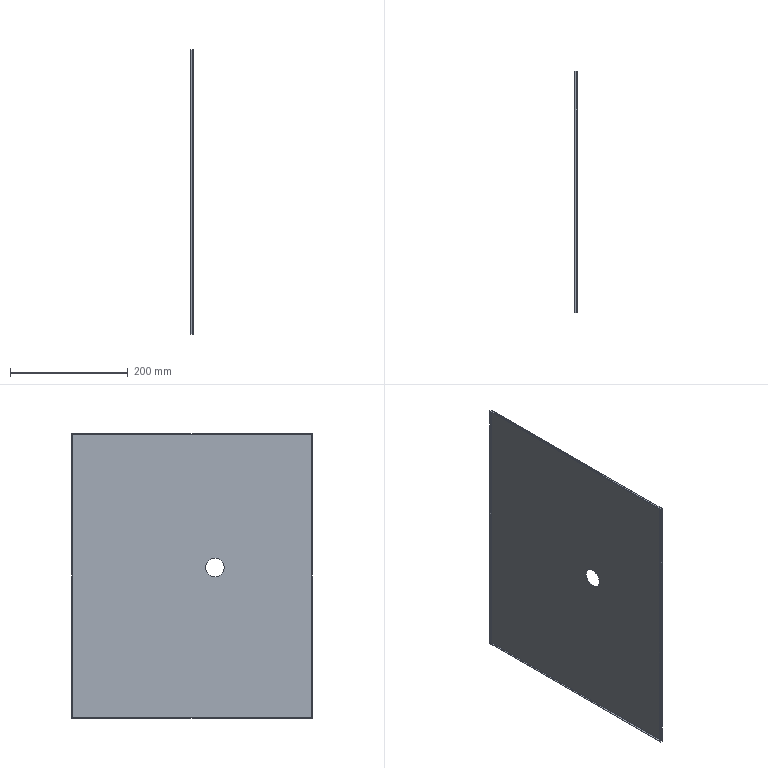Part | STEP file | 09-30 Cover base plate | 1 solid | 13 faces | box 4 x 410 x 485 mm | volume 203404 mm3 | plane 11 | cylinder 2 | commonest cylinder face diameters 32 x2
STEP:
#1=CARTESIAN_POINT('',(0.,0.,0.));
#2=DIRECTION('',(0.,0.,1.));
#3=DIRECTION('',(1.,0.,0.));
#4=AXIS2_PLACEMENT_3D('',#1,#2,#3);
#5=CARTESIAN_POINT('',(1.,-39.,30.5));
#6=VERTEX_POINT('',#5);
#7=CARTESIAN_POINT('',(0.,-39.,30.5));
#8=VERTEX_POINT('',#7);
#9=CARTESIAN_POINT('',(1.,-39.,30.5));
#10=DIRECTION('',(-1.,0.,0.));
#11=VECTOR('',#10,1.);
#12=LINE('',#9,#11);
#13=CARTESIAN_POINT('',(1.,-39.,14.5));
#14=DIRECTION('',(-1.,0.,0.));
#15=DIRECTION('',(0.,0.,1.));
#16=AXIS2_PLACEMENT_3D('',#13,#14,#15);
#17=CYLINDRICAL_SURFACE('',#16,16.);
#18=CARTESIAN_POINT('',(6.283,0.));
#19=DIRECTION('',(0.,1.));
#20=VECTOR('',#19,1.);
#21=LINE('',#18,#20);
#22=(GEOMETRIC_REPRESENTATION_CONTEXT(2)PARAMETRIC_REPRESENTATION_CONTEXT()REPRESENTATION_CONTEXT('',''));
#23=DEFINITIONAL_REPRESENTATION('',(#21),#22);
#24=PCURVE('',#17,#23);
#25=CARTESIAN_POINT('',(1.,-39.,14.5));
#26=DIRECTION('',(-1.,0.,0.));
#27=DIRECTION('',(0.,0.,1.));
#28=AXIS2_PLACEMENT_3D('',#25,#26,#27);
#29=CYLINDRICAL_SURFACE('',#28,16.);
#30=CARTESIAN_POINT('',(0.,0.));
#31=DIRECTION('',(0.,1.));
#32=VECTOR('',#31,1.);
#33=LINE('',#30,#32);
#34=(GEOMETRIC_REPRESENTATION_CONTEXT(2)PARAMETRIC_REPRESENTATION_CONTEXT()REPRESENTATION_CONTEXT('',''));
#35=DEFINITIONAL_REPRESENTATION('',(#33),#34);
#36=PCURVE('',#29,#35);
#37=SURFACE_CURVE('',#12,(#24,#36),.PCURVE_S1.);
#38=EDGE_CURVE('',#6,#8,#37,.T.);
#39=ORIENTED_EDGE('',*,*,#38,.T.);
#40=CARTESIAN_POINT('',(0.,-39.,-1.5));
#41=VERTEX_POINT('',#40);
#42=CARTESIAN_POINT('',(0.,-39.,14.5));
#43=DIRECTION('',(-1.,0.,0.));
#44=DIRECTION('',(0.,0.,1.));
#45=AXIS2_PLACEMENT_3D('',#42,#43,#44);
#46=CIRCLE('',#45,16.);
#47=CARTESIAN_POINT('',(0.,1.));
#48=DIRECTION('',(1.,0.));
#49=VECTOR('',#48,1.);
#50=LINE('',#47,#49);
#51=(GEOMETRIC_REPRESENTATION_CONTEXT(2)PARAMETRIC_REPRESENTATION_CONTEXT()REPRESENTATION_CONTEXT('',''));
#52=DEFINITIONAL_REPRESENTATION('',(#50),#51);
#53=PCURVE('',#17,#52);
#54=CARTESIAN_POINT('',(0.,-204.,-241.5));
#55=DIRECTION('',(-1.,0.,0.));
#56=DIRECTION('',(0.,0.,1.));
#57=AXIS2_PLACEMENT_3D('',#54,#55,#56);
#58=PLANE('',#57);
#59=CARTESIAN_POINT('',(256.,165.));
#60=DIRECTION('',(1.,0.));
#61=AXIS2_PLACEMENT_2D('',#59,#60);
#62=CIRCLE('',#61,16.);
#63=(GEOMETRIC_REPRESENTATION_CONTEXT(2)PARAMETRIC_REPRESENTATION_CONTEXT()REPRESENTATION_CONTEXT('',''));
#64=DEFINITIONAL_REPRESENTATION('',(#62),#63);
#65=PCURVE('',#58,#64);
#66=SURFACE_CURVE('',#46,(#53,#65),.PCURVE_S1.);
#67=EDGE_CURVE('',#41,#8,#66,.T.);
#68=ORIENTED_EDGE('',*,*,#67,.F.);
#69=CARTESIAN_POINT('',(1.,-39.,-1.5));
#70=VERTEX_POINT('',#69);
#71=CARTESIAN_POINT('',(1.,-39.,-1.5));
#72=DIRECTION('',(-1.,0.,0.));
#73=VECTOR('',#72,1.);
#74=LINE('',#71,#73);
#75=CARTESIAN_POINT('',(3.142,0.));
#76=DIRECTION('',(0.,1.));
#77=VECTOR('',#76,1.);
#78=LINE('',#75,#77);
#79=(GEOMETRIC_REPRESENTATION_CONTEXT(2)PARAMETRIC_REPRESENTATION_CONTEXT()REPRESENTATION_CONTEXT('',''));
#80=DEFINITIONAL_REPRESENTATION('',(#78),#79);
#81=PCURVE('',#17,#80);
#82=CARTESIAN_POINT('',(3.142,0.));
#83=DIRECTION('',(0.,1.));
#84=VECTOR('',#83,1.);
#85=LINE('',#82,#84);
#86=(GEOMETRIC_REPRESENTATION_CONTEXT(2)PARAMETRIC_REPRESENTATION_CONTEXT()REPRESENTATION_CONTEXT('',''));
#87=DEFINITIONAL_REPRESENTATION('',(#85),#86);
#88=PCURVE('',#29,#87);
#89=SURFACE_CURVE('',#74,(#81,#88),.PCURVE_S1.);
#90=EDGE_CURVE('',#70,#41,#89,.T.);
#91=ORIENTED_EDGE('',*,*,#90,.F.);
#92=CARTESIAN_POINT('',(1.,-39.,14.5));
#93=DIRECTION('',(1.,0.,0.));
#94=DIRECTION('',(0.,0.,1.));
#95=AXIS2_PLACEMENT_3D('',#92,#93,#94);
#96=CIRCLE('',#95,16.);
#97=CARTESIAN_POINT('',(6.283,0.));
#98=DIRECTION('',(-1.,0.));
#99=VECTOR('',#98,1.);
#100=LINE('',#97,#99);
#101=(GEOMETRIC_REPRESENTATION_CONTEXT(2)PARAMETRIC_REPRESENTATION_CONTEXT()REPRESENTATION_CONTEXT('',''));
#102=DEFINITIONAL_REPRESENTATION('',(#100),#101);
#103=PCURVE('',#17,#102);
#104=CARTESIAN_POINT('',(1.,-205.,-242.5));
#105=DIRECTION('',(-1.,0.,0.));
#106=DIRECTION('',(0.,0.,1.));
#107=AXIS2_PLACEMENT_3D('',#104,#105,#106);
#108=PLANE('',#107);
#109=CARTESIAN_POINT('',(273.,166.));
#110=CARTESIAN_POINT('',(273.,138.287));
#111=CARTESIAN_POINT('',(249.,152.144));
#112=CARTESIAN_POINT('',(225.,166.));
#113=CARTESIAN_POINT('',(249.,179.856));
#114=CARTESIAN_POINT('',(273.,193.713));
#115=CARTESIAN_POINT('',(273.,166.));
#116=(BOUNDED_CURVE()B_SPLINE_CURVE(2,(#109,#110,#111,#112,#113,#114,#115),.UNSPECIFIED.,.T.,.F.)B_SPLINE_CURVE_WITH_KNOTS((1,2,2,2,2,1),(-2.094,0.,2.094,4.189,6.283,8.378),.UNSPECIFIED.)CURVE()GEOMETRIC_REPRESENTATION_ITEM()RATIONAL_B_SPLINE_CURVE((1.,0.5,1.,0.5,1.,0.5,1.))REPRESENTATION_ITEM(''));
#117=(GEOMETRIC_REPRESENTATION_CONTEXT(2)PARAMETRIC_REPRESENTATION_CONTEXT()REPRESENTATION_CONTEXT('',''));
#118=DEFINITIONAL_REPRESENTATION('',(#116),#117);
#119=PCURVE('',#108,#118);
#120=SURFACE_CURVE('',#96,(#103,#119),.PCURVE_S1.);
#121=EDGE_CURVE('',#6,#70,#120,.T.);
#122=ORIENTED_EDGE('',*,*,#121,.F.);
#123=EDGE_LOOP('',(#39,#68,#91,#122));
#124=FACE_BOUND('',#123,.F.);
#125=ADVANCED_FACE('',(#124),#17,.F.);
#126=CARTESIAN_POINT('',(0.,-39.,14.5));
#127=DIRECTION('',(-1.,0.,0.));
#128=DIRECTION('',(0.,0.,1.));
#129=AXIS2_PLACEMENT_3D('',#126,#127,#128);
#130=CIRCLE('',#129,16.);
#131=CARTESIAN_POINT('',(0.,1.));
#132=DIRECTION('',(1.,0.));
#133=VECTOR('',#132,1.);
#134=LINE('',#131,#133);
#135=(GEOMETRIC_REPRESENTATION_CONTEXT(2)PARAMETRIC_REPRESENTATION_CONTEXT()REPRESENTATION_CONTEXT('',''));
#136=DEFINITIONAL_REPRESENTATION('',(#134),#135);
#137=PCURVE('',#29,#136);
#138=CARTESIAN_POINT('',(256.,165.));
#139=DIRECTION('',(1.,0.));
#140=AXIS2_PLACEMENT_2D('',#138,#139);
#141=CIRCLE('',#140,16.);
#142=(GEOMETRIC_REPRESENTATION_CONTEXT(2)PARAMETRIC_REPRESENTATION_CONTEXT()REPRESENTATION_CONTEXT('',''));
#143=DEFINITIONAL_REPRESENTATION('',(#141),#142);
#144=PCURVE('',#58,#143);
#145=SURFACE_CURVE('',#130,(#137,#144),.PCURVE_S1.);
#146=EDGE_CURVE('',#8,#41,#145,.T.);
#147=ORIENTED_EDGE('',*,*,#146,.F.);
#148=ORIENTED_EDGE('',*,*,#38,.F.);
#149=CARTESIAN_POINT('',(1.,-39.,14.5));
#150=DIRECTION('',(1.,0.,0.));
#151=DIRECTION('',(0.,0.,1.));
#152=AXIS2_PLACEMENT_3D('',#149,#150,#151);
#153=CIRCLE('',#152,16.);
#154=CARTESIAN_POINT('',(6.283,0.));
#155=DIRECTION('',(-1.,0.));
#156=VECTOR('',#155,1.);
#157=LINE('',#154,#156);
#158=(GEOMETRIC_REPRESENTATION_CONTEXT(2)PARAMETRIC_REPRESENTATION_CONTEXT()REPRESENTATION_CONTEXT('',''));
#159=DEFINITIONAL_REPRESENTATION('',(#157),#158);
#160=PCURVE('',#29,#159);
#161=CARTESIAN_POINT('',(273.,166.));
#162=CARTESIAN_POINT('',(273.,138.287));
#163=CARTESIAN_POINT('',(249.,152.144));
#164=CARTESIAN_POINT('',(225.,166.));
#165=CARTESIAN_POINT('',(249.,179.856));
#166=CARTESIAN_POINT('',(273.,193.713));
#167=CARTESIAN_POINT('',(273.,166.));
#168=(BOUNDED_CURVE()B_SPLINE_CURVE(2,(#161,#162,#163,#164,#165,#166,#167),.UNSPECIFIED.,.T.,.F.)B_SPLINE_CURVE_WITH_KNOTS((1,2,2,2,2,1),(-2.094,0.,2.094,4.189,6.283,8.378),.UNSPECIFIED.)CURVE()GEOMETRIC_REPRESENTATION_ITEM()RATIONAL_B_SPLINE_CURVE((1.,0.5,1.,0.5,1.,0.5,1.))REPRESENTATION_ITEM(''));
#169=(GEOMETRIC_REPRESENTATION_CONTEXT(2)PARAMETRIC_REPRESENTATION_CONTEXT()REPRESENTATION_CONTEXT('',''));
#170=DEFINITIONAL_REPRESENTATION('',(#168),#169);
#171=PCURVE('',#108,#170);
#172=SURFACE_CURVE('',#153,(#160,#171),.PCURVE_S1.);
#173=EDGE_CURVE('',#70,#6,#172,.T.);
#174=ORIENTED_EDGE('',*,*,#173,.F.);
#175=ORIENTED_EDGE('',*,*,#90,.T.);
#176=EDGE_LOOP('',(#147,#148,#174,#175));
#177=FACE_BOUND('',#176,.F.);
#178=ADVANCED_FACE('',(#177),#29,.F.);
#179=ORIENTED_EDGE('',*,*,#146,.F.);
#180=ORIENTED_EDGE('',*,*,#67,.F.);
#181=EDGE_LOOP('',(#179,#180));
#182=FACE_BOUND('',#181,.T.);
#183=CARTESIAN_POINT('',(0.,204.,-241.5));
#184=VERTEX_POINT('',#183);
#185=CARTESIAN_POINT('',(0.,-204.,-241.5));
#186=VERTEX_POINT('',#185);
#187=CARTESIAN_POINT('',(0.,0.,-241.5));
#188=DIRECTION('',(0.,-1.,0.));
#189=VECTOR('',#188,1.);
#190=LINE('',#187,#189);
#191=CARTESIAN_POINT('',(0.,204.));
#192=DIRECTION('',(0.,-1.));
#193=VECTOR('',#192,1.);
#194=LINE('',#191,#193);
#195=(GEOMETRIC_REPRESENTATION_CONTEXT(2)PARAMETRIC_REPRESENTATION_CONTEXT()REPRESENTATION_CONTEXT('',''));
#196=DEFINITIONAL_REPRESENTATION('',(#194),#195);
#197=PCURVE('',#58,#196);
#198=CARTESIAN_POINT('',(-3.,-204.,-241.5));
#199=DIRECTION('',(0.,0.,1.));
#200=DIRECTION('',(1.,0.,0.));
#201=AXIS2_PLACEMENT_3D('',#198,#199,#200);
#202=PLANE('',#201);
#203=CARTESIAN_POINT('',(3.,204.));
#204=DIRECTION('',(0.,-1.));
#205=VECTOR('',#204,1.);
#206=LINE('',#203,#205);
#207=(GEOMETRIC_REPRESENTATION_CONTEXT(2)PARAMETRIC_REPRESENTATION_CONTEXT()REPRESENTATION_CONTEXT('',''));
#208=DEFINITIONAL_REPRESENTATION('',(#206),#207);
#209=PCURVE('',#202,#208);
#210=SURFACE_CURVE('',#190,(#197,#209),.PCURVE_S1.);
#211=EDGE_CURVE('',#184,#186,#210,.T.);
#212=ORIENTED_EDGE('',*,*,#211,.T.);
#213=CARTESIAN_POINT('',(0.,-204.,241.5));
#214=VERTEX_POINT('',#213);
#215=CARTESIAN_POINT('',(0.,-204.,0.));
#216=DIRECTION('',(0.,0.,1.));
#217=VECTOR('',#216,1.);
#218=LINE('',#215,#217);
#219=CARTESIAN_POINT('',(241.5,0.));
#220=DIRECTION('',(1.,0.));
#221=VECTOR('',#220,1.);
#222=LINE('',#219,#221);
#223=(GEOMETRIC_REPRESENTATION_CONTEXT(2)PARAMETRIC_REPRESENTATION_CONTEXT()REPRESENTATION_CONTEXT('',''));
#224=DEFINITIONAL_REPRESENTATION('',(#222),#223);
#225=PCURVE('',#58,#224);
#226=CARTESIAN_POINT('',(-3.,-204.,-241.5));
#227=DIRECTION('',(0.,1.,0.));
#228=DIRECTION('',(0.,0.,1.));
#229=AXIS2_PLACEMENT_3D('',#226,#227,#228);
#230=PLANE('',#229);
#231=CARTESIAN_POINT('',(241.5,3.));
#232=DIRECTION('',(1.,0.));
#233=VECTOR('',#232,1.);
#234=LINE('',#231,#233);
#235=(GEOMETRIC_REPRESENTATION_CONTEXT(2)PARAMETRIC_REPRESENTATION_CONTEXT()REPRESENTATION_CONTEXT('',''));
#236=DEFINITIONAL_REPRESENTATION('',(#234),#235);
#237=PCURVE('',#230,#236);
#238=SURFACE_CURVE('',#218,(#225,#237),.PCURVE_S1.);
#239=EDGE_CURVE('',#186,#214,#238,.T.);
#240=ORIENTED_EDGE('',*,*,#239,.T.);
#241=CARTESIAN_POINT('',(0.,204.,241.5));
#242=VERTEX_POINT('',#241);
#243=CARTESIAN_POINT('',(0.,0.,241.5));
#244=DIRECTION('',(0.,1.,0.));
#245=VECTOR('',#244,1.);
#246=LINE('',#243,#245);
#247=CARTESIAN_POINT('',(483.,204.));
#248=DIRECTION('',(0.,1.));
#249=VECTOR('',#248,1.);
#250=LINE('',#247,#249);
#251=(GEOMETRIC_REPRESENTATION_CONTEXT(2)PARAMETRIC_REPRESENTATION_CONTEXT()REPRESENTATION_CONTEXT('',''));
#252=DEFINITIONAL_REPRESENTATION('',(#250),#251);
#253=PCURVE('',#58,#252);
#254=CARTESIAN_POINT('',(0.,-204.,241.5));
#255=DIRECTION('',(0.,0.,-1.));
#256=DIRECTION('',(-1.,0.,0.));
#257=AXIS2_PLACEMENT_3D('',#254,#255,#256);
#258=PLANE('',#257);
#259=CARTESIAN_POINT('',(0.,204.));
#260=DIRECTION('',(0.,1.));
#261=VECTOR('',#260,1.);
#262=LINE('',#259,#261);
#263=(GEOMETRIC_REPRESENTATION_CONTEXT(2)PARAMETRIC_REPRESENTATION_CONTEXT()REPRESENTATION_CONTEXT('',''));
#264=DEFINITIONAL_REPRESENTATION('',(#262),#263);
#265=PCURVE('',#258,#264);
#266=SURFACE_CURVE('',#246,(#253,#265),.PCURVE_S1.);
#267=EDGE_CURVE('',#214,#242,#266,.T.);
#268=ORIENTED_EDGE('',*,*,#267,.T.);
#269=CARTESIAN_POINT('',(0.,204.,0.));
#270=DIRECTION('',(0.,0.,-1.));
#271=VECTOR('',#270,1.);
#272=LINE('',#269,#271);
#273=CARTESIAN_POINT('',(241.5,408.));
#274=DIRECTION('',(-1.,0.));
#275=VECTOR('',#274,1.);
#276=LINE('',#273,#275);
#277=(GEOMETRIC_REPRESENTATION_CONTEXT(2)PARAMETRIC_REPRESENTATION_CONTEXT()REPRESENTATION_CONTEXT('',''));
#278=DEFINITIONAL_REPRESENTATION('',(#276),#277);
#279=PCURVE('',#58,#278);
#280=CARTESIAN_POINT('',(-3.,204.,241.5));
#281=DIRECTION('',(0.,-1.,0.));
#282=DIRECTION('',(0.,0.,-1.));
#283=AXIS2_PLACEMENT_3D('',#280,#281,#282);
#284=PLANE('',#283);
#285=CARTESIAN_POINT('',(241.5,3.));
#286=DIRECTION('',(1.,0.));
#287=VECTOR('',#286,1.);
#288=LINE('',#285,#287);
#289=(GEOMETRIC_REPRESENTATION_CONTEXT(2)PARAMETRIC_REPRESENTATION_CONTEXT()REPRESENTATION_CONTEXT('',''));
#290=DEFINITIONAL_REPRESENTATION('',(#288),#289);
#291=PCURVE('',#284,#290);
#292=SURFACE_CURVE('',#272,(#279,#291),.PCURVE_S1.);
#293=EDGE_CURVE('',#242,#184,#292,.T.);
#294=ORIENTED_EDGE('',*,*,#293,.T.);
#295=EDGE_LOOP('',(#212,#240,#268,#294));
#296=FACE_BOUND('',#295,.T.);
#297=ADVANCED_FACE('',(#182,#296),#58,.T.);
#298=ORIENTED_EDGE('',*,*,#121,.F.);
#299=ORIENTED_EDGE('',*,*,#173,.F.);
#300=EDGE_LOOP('',(#298,#299));
#301=FACE_BOUND('',#300,.T.);
#302=CARTESIAN_POINT('',(1.,205.,242.5));
#303=VERTEX_POINT('',#302);
#304=CARTESIAN_POINT('',(1.,205.,-242.5));
#305=VERTEX_POINT('',#304);
#306=CARTESIAN_POINT('',(1.,205.,0.));
#307=DIRECTION('',(0.,0.,-1.));
#308=VECTOR('',#307,1.);
#309=LINE('',#306,#308);
#310=CARTESIAN_POINT('',(242.5,410.));
#311=DIRECTION('',(-1.,0.));
#312=VECTOR('',#311,1.);
#313=LINE('',#310,#312);
#314=(GEOMETRIC_REPRESENTATION_CONTEXT(2)PARAMETRIC_REPRESENTATION_CONTEXT()REPRESENTATION_CONTEXT('',''));
#315=DEFINITIONAL_REPRESENTATION('',(#313),#314);
#316=PCURVE('',#108,#315);
#317=CARTESIAN_POINT('',(-3.,205.,242.5));
#318=DIRECTION('',(0.,-1.,0.));
#319=DIRECTION('',(0.,0.,-1.));
#320=AXIS2_PLACEMENT_3D('',#317,#318,#319);
#321=PLANE('',#320);
#322=CARTESIAN_POINT('',(242.5,4.));
#323=DIRECTION('',(1.,0.));
#324=VECTOR('',#323,1.);
#325=LINE('',#322,#324);
#326=(GEOMETRIC_REPRESENTATION_CONTEXT(2)PARAMETRIC_REPRESENTATION_CONTEXT()REPRESENTATION_CONTEXT('',''));
#327=DEFINITIONAL_REPRESENTATION('',(#325),#326);
#328=PCURVE('',#321,#327);
#329=SURFACE_CURVE('',#309,(#316,#328),.PCURVE_S1.);
#330=EDGE_CURVE('',#303,#305,#329,.T.);
#331=ORIENTED_EDGE('',*,*,#330,.F.);
#332=CARTESIAN_POINT('',(1.,-205.,242.5));
#333=VERTEX_POINT('',#332);
#334=CARTESIAN_POINT('',(1.,0.,242.5));
#335=DIRECTION('',(0.,1.,0.));
#336=VECTOR('',#335,1.);
#337=LINE('',#334,#336);
#338=CARTESIAN_POINT('',(485.,205.));
#339=DIRECTION('',(0.,1.));
#340=VECTOR('',#339,1.);
#341=LINE('',#338,#340);
#342=(GEOMETRIC_REPRESENTATION_CONTEXT(2)PARAMETRIC_REPRESENTATION_CONTEXT()REPRESENTATION_CONTEXT('',''));
#343=DEFINITIONAL_REPRESENTATION('',(#341),#342);
#344=PCURVE('',#108,#343);
#345=CARTESIAN_POINT('',(1.,-205.,242.5));
#346=DIRECTION('',(0.,0.,-1.));
#347=DIRECTION('',(-1.,0.,0.));
#348=AXIS2_PLACEMENT_3D('',#345,#346,#347);
#349=PLANE('',#348);
#350=CARTESIAN_POINT('',(0.,205.));
#351=DIRECTION('',(0.,1.));
#352=VECTOR('',#351,1.);
#353=LINE('',#350,#352);
#354=(GEOMETRIC_REPRESENTATION_CONTEXT(2)PARAMETRIC_REPRESENTATION_CONTEXT()REPRESENTATION_CONTEXT('',''));
#355=DEFINITIONAL_REPRESENTATION('',(#353),#354);
#356=PCURVE('',#349,#355);
#357=SURFACE_CURVE('',#337,(#344,#356),.PCURVE_S1.);
#358=EDGE_CURVE('',#333,#303,#357,.T.);
#359=ORIENTED_EDGE('',*,*,#358,.F.);
#360=CARTESIAN_POINT('',(1.,-205.,-242.5));
#361=VERTEX_POINT('',#360);
#362=CARTESIAN_POINT('',(1.,-205.,0.));
#363=DIRECTION('',(0.,0.,1.));
#364=VECTOR('',#363,1.);
#365=LINE('',#362,#364);
#366=CARTESIAN_POINT('',(242.5,0.));
#367=DIRECTION('',(1.,0.));
#368=VECTOR('',#367,1.);
#369=LINE('',#366,#368);
#370=(GEOMETRIC_REPRESENTATION_CONTEXT(2)PARAMETRIC_REPRESENTATION_CONTEXT()REPRESENTATION_CONTEXT('',''));
#371=DEFINITIONAL_REPRESENTATION('',(#369),#370);
#372=PCURVE('',#108,#371);
#373=CARTESIAN_POINT('',(-3.,-205.,-242.5));
#374=DIRECTION('',(0.,1.,0.));
#375=DIRECTION('',(0.,0.,1.));
#376=AXIS2_PLACEMENT_3D('',#373,#374,#375);
#377=PLANE('',#376);
#378=CARTESIAN_POINT('',(242.5,4.));
#379=DIRECTION('',(1.,0.));
#380=VECTOR('',#379,1.);
#381=LINE('',#378,#380);
#382=(GEOMETRIC_REPRESENTATION_CONTEXT(2)PARAMETRIC_REPRESENTATION_CONTEXT()REPRESENTATION_CONTEXT('',''));
#383=DEFINITIONAL_REPRESENTATION('',(#381),#382);
#384=PCURVE('',#377,#383);
#385=SURFACE_CURVE('',#365,(#372,#384),.PCURVE_S1.);
#386=EDGE_CURVE('',#361,#333,#385,.T.);
#387=ORIENTED_EDGE('',*,*,#386,.F.);
#388=CARTESIAN_POINT('',(1.,0.,-242.5));
#389=DIRECTION('',(0.,-1.,0.));
#390=VECTOR('',#389,1.);
#391=LINE('',#388,#390);
#392=CARTESIAN_POINT('',(0.,205.));
#393=DIRECTION('',(0.,-1.));
#394=VECTOR('',#393,1.);
#395=LINE('',#392,#394);
#396=(GEOMETRIC_REPRESENTATION_CONTEXT(2)PARAMETRIC_REPRESENTATION_CONTEXT()REPRESENTATION_CONTEXT('',''));
#397=DEFINITIONAL_REPRESENTATION('',(#395),#396);
#398=PCURVE('',#108,#397);
#399=CARTESIAN_POINT('',(-3.,-205.,-242.5));
#400=DIRECTION('',(0.,0.,1.));
#401=DIRECTION('',(1.,0.,0.));
#402=AXIS2_PLACEMENT_3D('',#399,#400,#401);
#403=PLANE('',#402);
#404=CARTESIAN_POINT('',(4.,205.));
#405=DIRECTION('',(0.,-1.));
#406=VECTOR('',#405,1.);
#407=LINE('',#404,#406);
#408=(GEOMETRIC_REPRESENTATION_CONTEXT(2)PARAMETRIC_REPRESENTATION_CONTEXT()REPRESENTATION_CONTEXT('',''));
#409=DEFINITIONAL_REPRESENTATION('',(#407),#408);
#410=PCURVE('',#403,#409);
#411=SURFACE_CURVE('',#391,(#398,#410),.PCURVE_S1.);
#412=EDGE_CURVE('',#305,#361,#411,.T.);
#413=ORIENTED_EDGE('',*,*,#412,.F.);
#414=EDGE_LOOP('',(#331,#359,#387,#413));
#415=FACE_BOUND('',#414,.T.);
#416=ADVANCED_FACE('',(#301,#415),#108,.F.);
#417=CARTESIAN_POINT('',(-3.,-204.,-241.5));
#418=VERTEX_POINT('',#417);
#419=CARTESIAN_POINT('',(-3.,-204.,241.5));
#420=VERTEX_POINT('',#419);
#421=CARTESIAN_POINT('',(-3.,-204.,0.));
#422=DIRECTION('',(0.,0.,1.));
#423=VECTOR('',#422,1.);
#424=LINE('',#421,#423);
#425=CARTESIAN_POINT('',(241.5,0.));
#426=DIRECTION('',(1.,0.));
#427=VECTOR('',#426,1.);
#428=LINE('',#425,#427);
#429=(GEOMETRIC_REPRESENTATION_CONTEXT(2)PARAMETRIC_REPRESENTATION_CONTEXT()REPRESENTATION_CONTEXT('',''));
#430=DEFINITIONAL_REPRESENTATION('',(#428),#429);
#431=PCURVE('',#230,#430);
#432=CARTESIAN_POINT('',(-3.,-205.,242.5));
#433=DIRECTION('',(1.,0.,0.));
#434=DIRECTION('',(0.,0.,-1.));
#435=AXIS2_PLACEMENT_3D('',#432,#433,#434);
#436=PLANE('',#435);
#437=CARTESIAN_POINT('',(242.5,1.));
#438=DIRECTION('',(-1.,0.));
#439=VECTOR('',#438,1.);
#440=LINE('',#437,#439);
#441=(GEOMETRIC_REPRESENTATION_CONTEXT(2)PARAMETRIC_REPRESENTATION_CONTEXT()REPRESENTATION_CONTEXT('',''));
#442=DEFINITIONAL_REPRESENTATION('',(#440),#441);
#443=PCURVE('',#436,#442);
#444=SURFACE_CURVE('',#424,(#431,#443),.PCURVE_S1.);
#445=EDGE_CURVE('',#418,#420,#444,.T.);
#446=ORIENTED_EDGE('',*,*,#445,.T.);
#447=CARTESIAN_POINT('',(-1.5,-204.,241.5));
#448=DIRECTION('',(1.,0.,0.));
#449=VECTOR('',#448,1.);
#450=LINE('',#447,#449);
#451=CARTESIAN_POINT('',(483.,1.5));
#452=DIRECTION('',(0.,1.));
#453=VECTOR('',#452,1.);
#454=LINE('',#451,#453);
#455=(GEOMETRIC_REPRESENTATION_CONTEXT(2)PARAMETRIC_REPRESENTATION_CONTEXT()REPRESENTATION_CONTEXT('',''));
#456=DEFINITIONAL_REPRESENTATION('',(#454),#455);
#457=PCURVE('',#230,#456);
#458=CARTESIAN_POINT('',(1.5,0.));
#459=DIRECTION('',(-1.,0.));
#460=VECTOR('',#459,1.);
#461=LINE('',#458,#460);
#462=(GEOMETRIC_REPRESENTATION_CONTEXT(2)PARAMETRIC_REPRESENTATION_CONTEXT()REPRESENTATION_CONTEXT('',''));
#463=DEFINITIONAL_REPRESENTATION('',(#461),#462);
#464=PCURVE('',#258,#463);
#465=SURFACE_CURVE('',#450,(#457,#464),.PCURVE_S1.);
#466=EDGE_CURVE('',#420,#214,#465,.T.);
#467=ORIENTED_EDGE('',*,*,#466,.T.);
#468=ORIENTED_EDGE('',*,*,#239,.F.);
#469=CARTESIAN_POINT('',(-1.5,-204.,-241.5));
#470=DIRECTION('',(-1.,0.,0.));
#471=VECTOR('',#470,1.);
#472=LINE('',#469,#471);
#473=CARTESIAN_POINT('',(0.,1.5));
#474=DIRECTION('',(0.,-1.));
#475=VECTOR('',#474,1.);
#476=LINE('',#473,#475);
#477=(GEOMETRIC_REPRESENTATION_CONTEXT(2)PARAMETRIC_REPRESENTATION_CONTEXT()REPRESENTATION_CONTEXT('',''));
#478=DEFINITIONAL_REPRESENTATION('',(#476),#477);
#479=PCURVE('',#230,#478);
#480=CARTESIAN_POINT('',(1.5,0.));
#481=DIRECTION('',(-1.,0.));
#482=VECTOR('',#481,1.);
#483=LINE('',#480,#482);
#484=(GEOMETRIC_REPRESENTATION_CONTEXT(2)PARAMETRIC_REPRESENTATION_CONTEXT()REPRESENTATION_CONTEXT('',''));
#485=DEFINITIONAL_REPRESENTATION('',(#483),#484);
#486=PCURVE('',#202,#485);
#487=SURFACE_CURVE('',#472,(#479,#486),.PCURVE_S1.);
#488=EDGE_CURVE('',#186,#418,#487,.T.);
#489=ORIENTED_EDGE('',*,*,#488,.T.);
#490=EDGE_LOOP('',(#446,#467,#468,#489));
#491=FACE_BOUND('',#490,.T.);
#492=ADVANCED_FACE('',(#491),#230,.T.);
#493=CARTESIAN_POINT('',(-3.,204.,-241.5));
#494=VERTEX_POINT('',#493);
#495=CARTESIAN_POINT('',(-3.,0.,-241.5));
#496=DIRECTION('',(0.,-1.,0.));
#497=VECTOR('',#496,1.);
#498=LINE('',#495,#497);
#499=CARTESIAN_POINT('',(0.,204.));
#500=DIRECTION('',(0.,-1.));
#501=VECTOR('',#500,1.);
#502=LINE('',#499,#501);
#503=(GEOMETRIC_REPRESENTATION_CONTEXT(2)PARAMETRIC_REPRESENTATION_CONTEXT()REPRESENTATION_CONTEXT('',''));
#504=DEFINITIONAL_REPRESENTATION('',(#502),#503);
#505=PCURVE('',#202,#504);
#506=CARTESIAN_POINT('',(484.,205.));
#507=DIRECTION('',(0.,-1.));
#508=VECTOR('',#507,1.);
#509=LINE('',#506,#508);
#510=(GEOMETRIC_REPRESENTATION_CONTEXT(2)PARAMETRIC_REPRESENTATION_CONTEXT()REPRESENTATION_CONTEXT('',''));
#511=DEFINITIONAL_REPRESENTATION('',(#509),#510);
#512=PCURVE('',#436,#511);
#513=SURFACE_CURVE('',#498,(#505,#512),.PCURVE_S1.);
#514=EDGE_CURVE('',#494,#418,#513,.T.);
#515=ORIENTED_EDGE('',*,*,#514,.T.);
#516=ORIENTED_EDGE('',*,*,#488,.F.);
#517=ORIENTED_EDGE('',*,*,#211,.F.);
#518=CARTESIAN_POINT('',(-1.5,204.,-241.5));
#519=DIRECTION('',(-1.,0.,0.));
#520=VECTOR('',#519,1.);
#521=LINE('',#518,#520);
#522=CARTESIAN_POINT('',(1.5,408.));
#523=DIRECTION('',(-1.,0.));
#524=VECTOR('',#523,1.);
#525=LINE('',#522,#524);
#526=(GEOMETRIC_REPRESENTATION_CONTEXT(2)PARAMETRIC_REPRESENTATION_CONTEXT()REPRESENTATION_CONTEXT('',''));
#527=DEFINITIONAL_REPRESENTATION('',(#525),#526);
#528=PCURVE('',#202,#527);
#529=CARTESIAN_POINT('',(483.,1.5));
#530=DIRECTION('',(0.,-1.));
#531=VECTOR('',#530,1.);
#532=LINE('',#529,#531);
#533=(GEOMETRIC_REPRESENTATION_CONTEXT(2)PARAMETRIC_REPRESENTATION_CONTEXT()REPRESENTATION_CONTEXT('',''));
#534=DEFINITIONAL_REPRESENTATION('',(#532),#533);
#535=PCURVE('',#284,#534);
#536=SURFACE_CURVE('',#521,(#528,#535),.PCURVE_S1.);
#537=EDGE_CURVE('',#184,#494,#536,.T.);
#538=ORIENTED_EDGE('',*,*,#537,.T.);
#539=EDGE_LOOP('',(#515,#516,#517,#538));
#540=FACE_BOUND('',#539,.T.);
#541=ADVANCED_FACE('',(#540),#202,.T.);
#542=CARTESIAN_POINT('',(-3.,204.,241.5));
#543=VERTEX_POINT('',#542);
#544=CARTESIAN_POINT('',(-3.,204.,0.));
#545=DIRECTION('',(0.,0.,-1.));
#546=VECTOR('',#545,1.);
#547=LINE('',#544,#546);
#548=CARTESIAN_POINT('',(241.5,0.));
#549=DIRECTION('',(1.,0.));
#550=VECTOR('',#549,1.);
#551=LINE('',#548,#550);
#552=(GEOMETRIC_REPRESENTATION_CONTEXT(2)PARAMETRIC_REPRESENTATION_CONTEXT()REPRESENTATION_CONTEXT('',''));
#553=DEFINITIONAL_REPRESENTATION('',(#551),#552);
#554=PCURVE('',#284,#553);
#555=CARTESIAN_POINT('',(242.5,409.));
#556=DIRECTION('',(1.,0.));
#557=VECTOR('',#556,1.);
#558=LINE('',#555,#557);
#559=(GEOMETRIC_REPRESENTATION_CONTEXT(2)PARAMETRIC_REPRESENTATION_CONTEXT()REPRESENTATION_CONTEXT('',''));
#560=DEFINITIONAL_REPRESENTATION('',(#558),#559);
#561=PCURVE('',#436,#560);
#562=SURFACE_CURVE('',#547,(#554,#561),.PCURVE_S1.);
#563=EDGE_CURVE('',#543,#494,#562,.T.);
#564=ORIENTED_EDGE('',*,*,#563,.T.);
#565=ORIENTED_EDGE('',*,*,#537,.F.);
#566=ORIENTED_EDGE('',*,*,#293,.F.);
#567=CARTESIAN_POINT('',(-1.5,204.,241.5));
#568=DIRECTION('',(-1.,0.,0.));
#569=VECTOR('',#568,1.);
#570=LINE('',#567,#569);
#571=CARTESIAN_POINT('',(0.,1.5));
#572=DIRECTION('',(0.,-1.));
#573=VECTOR('',#572,1.);
#574=LINE('',#571,#573);
#575=(GEOMETRIC_REPRESENTATION_CONTEXT(2)PARAMETRIC_REPRESENTATION_CONTEXT()REPRESENTATION_CONTEXT('',''));
#576=DEFINITIONAL_REPRESENTATION('',(#574),#575);
#577=PCURVE('',#284,#576);
#578=CARTESIAN_POINT('',(1.5,408.));
#579=DIRECTION('',(1.,0.));
#580=VECTOR('',#579,1.);
#581=LINE('',#578,#580);
#582=(GEOMETRIC_REPRESENTATION_CONTEXT(2)PARAMETRIC_REPRESENTATION_CONTEXT()REPRESENTATION_CONTEXT('',''));
#583=DEFINITIONAL_REPRESENTATION('',(#581),#582);
#584=PCURVE('',#258,#583);
#585=SURFACE_CURVE('',#570,(#577,#584),.PCURVE_S1.);
#586=EDGE_CURVE('',#242,#543,#585,.T.);
#587=ORIENTED_EDGE('',*,*,#586,.T.);
#588=EDGE_LOOP('',(#564,#565,#566,#587));
#589=FACE_BOUND('',#588,.T.);
#590=ADVANCED_FACE('',(#589),#284,.T.);
#591=CARTESIAN_POINT('',(-3.,0.,241.5));
#592=DIRECTION('',(0.,1.,0.));
#593=VECTOR('',#592,1.);
#594=LINE('',#591,#593);
#595=CARTESIAN_POINT('',(3.,204.));
#596=DIRECTION('',(0.,1.));
#597=VECTOR('',#596,1.);
#598=LINE('',#595,#597);
#599=(GEOMETRIC_REPRESENTATION_CONTEXT(2)PARAMETRIC_REPRESENTATION_CONTEXT()REPRESENTATION_CONTEXT('',''));
#600=DEFINITIONAL_REPRESENTATION('',(#598),#599);
#601=PCURVE('',#258,#600);
#602=CARTESIAN_POINT('',(1.,205.));
#603=DIRECTION('',(0.,1.));
#604=VECTOR('',#603,1.);
#605=LINE('',#602,#604);
#606=(GEOMETRIC_REPRESENTATION_CONTEXT(2)PARAMETRIC_REPRESENTATION_CONTEXT()REPRESENTATION_CONTEXT('',''));
#607=DEFINITIONAL_REPRESENTATION('',(#605),#606);
#608=PCURVE('',#436,#607);
#609=SURFACE_CURVE('',#594,(#601,#608),.PCURVE_S1.);
#610=EDGE_CURVE('',#420,#543,#609,.T.);
#611=ORIENTED_EDGE('',*,*,#610,.T.);
#612=ORIENTED_EDGE('',*,*,#586,.F.);
#613=ORIENTED_EDGE('',*,*,#267,.F.);
#614=ORIENTED_EDGE('',*,*,#466,.F.);
#615=EDGE_LOOP('',(#611,#612,#613,#614));
#616=FACE_BOUND('',#615,.T.);
#617=ADVANCED_FACE('',(#616),#258,.T.);
#618=CARTESIAN_POINT('',(-3.,205.,-242.5));
#619=VERTEX_POINT('',#618);
#620=CARTESIAN_POINT('',(-3.,-205.,-242.5));
#621=VERTEX_POINT('',#620);
#622=CARTESIAN_POINT('',(-3.,0.,-242.5));
#623=DIRECTION('',(0.,-1.,0.));
#624=VECTOR('',#623,1.);
#625=LINE('',#622,#624);
#626=CARTESIAN_POINT('',(0.,205.));
#627=DIRECTION('',(0.,-1.));
#628=VECTOR('',#627,1.);
#629=LINE('',#626,#628);
#630=(GEOMETRIC_REPRESENTATION_CONTEXT(2)PARAMETRIC_REPRESENTATION_CONTEXT()REPRESENTATION_CONTEXT('',''));
#631=DEFINITIONAL_REPRESENTATION('',(#629),#630);
#632=PCURVE('',#403,#631);
#633=CARTESIAN_POINT('',(485.,205.));
#634=DIRECTION('',(0.,-1.));
#635=VECTOR('',#634,1.);
#636=LINE('',#633,#635);
#637=(GEOMETRIC_REPRESENTATION_CONTEXT(2)PARAMETRIC_REPRESENTATION_CONTEXT()REPRESENTATION_CONTEXT('',''));
#638=DEFINITIONAL_REPRESENTATION('',(#636),#637);
#639=PCURVE('',#436,#638);
#640=SURFACE_CURVE('',#625,(#632,#639),.PCURVE_S1.);
#641=EDGE_CURVE('',#619,#621,#640,.T.);
#642=ORIENTED_EDGE('',*,*,#641,.F.);
#643=CARTESIAN_POINT('',(-1.,205.,-242.5));
#644=DIRECTION('',(-1.,0.,0.));
#645=VECTOR('',#644,1.);
#646=LINE('',#643,#645);
#647=CARTESIAN_POINT('',(2.,410.));
#648=DIRECTION('',(-1.,0.));
#649=VECTOR('',#648,1.);
#650=LINE('',#647,#649);
#651=(GEOMETRIC_REPRESENTATION_CONTEXT(2)PARAMETRIC_REPRESENTATION_CONTEXT()REPRESENTATION_CONTEXT('',''));
#652=DEFINITIONAL_REPRESENTATION('',(#650),#651);
#653=PCURVE('',#403,#652);
#654=CARTESIAN_POINT('',(485.,2.));
#655=DIRECTION('',(0.,-1.));
#656=VECTOR('',#655,1.);
#657=LINE('',#654,#656);
#658=(GEOMETRIC_REPRESENTATION_CONTEXT(2)PARAMETRIC_REPRESENTATION_CONTEXT()REPRESENTATION_CONTEXT('',''));
#659=DEFINITIONAL_REPRESENTATION('',(#657),#658);
#660=PCURVE('',#321,#659);
#661=SURFACE_CURVE('',#646,(#653,#660),.PCURVE_S1.);
#662=EDGE_CURVE('',#305,#619,#661,.T.);
#663=ORIENTED_EDGE('',*,*,#662,.F.);
#664=ORIENTED_EDGE('',*,*,#412,.T.);
#665=CARTESIAN_POINT('',(-1.,-205.,-242.5));
#666=DIRECTION('',(1.,0.,0.));
#667=VECTOR('',#666,1.);
#668=LINE('',#665,#667);
#669=CARTESIAN_POINT('',(2.,0.));
#670=DIRECTION('',(1.,0.));
#671=VECTOR('',#670,1.);
#672=LINE('',#669,#671);
#673=(GEOMETRIC_REPRESENTATION_CONTEXT(2)PARAMETRIC_REPRESENTATION_CONTEXT()REPRESENTATION_CONTEXT('',''));
#674=DEFINITIONAL_REPRESENTATION('',(#672),#673);
#675=PCURVE('',#403,#674);
#676=CARTESIAN_POINT('',(0.,2.));
#677=DIRECTION('',(0.,1.));
#678=VECTOR('',#677,1.);
#679=LINE('',#676,#678);
#680=(GEOMETRIC_REPRESENTATION_CONTEXT(2)PARAMETRIC_REPRESENTATION_CONTEXT()REPRESENTATION_CONTEXT('',''));
#681=DEFINITIONAL_REPRESENTATION('',(#679),#680);
#682=PCURVE('',#377,#681);
#683=SURFACE_CURVE('',#668,(#675,#682),.PCURVE_S1.);
#684=EDGE_CURVE('',#621,#361,#683,.T.);
#685=ORIENTED_EDGE('',*,*,#684,.F.);
#686=EDGE_LOOP('',(#642,#663,#664,#685));
#687=FACE_BOUND('',#686,.T.);
#688=ADVANCED_FACE('',(#687),#403,.F.);
#689=CARTESIAN_POINT('',(-3.,205.,242.5));
#690=VERTEX_POINT('',#689);
#691=CARTESIAN_POINT('',(-3.,205.,0.));
#692=DIRECTION('',(0.,0.,-1.));
#693=VECTOR('',#692,1.);
#694=LINE('',#691,#693);
#695=CARTESIAN_POINT('',(242.5,0.));
#696=DIRECTION('',(1.,0.));
#697=VECTOR('',#696,1.);
#698=LINE('',#695,#697);
#699=(GEOMETRIC_REPRESENTATION_CONTEXT(2)PARAMETRIC_REPRESENTATION_CONTEXT()REPRESENTATION_CONTEXT('',''));
#700=DEFINITIONAL_REPRESENTATION('',(#698),#699);
#701=PCURVE('',#321,#700);
#702=CARTESIAN_POINT('',(242.5,410.));
#703=DIRECTION('',(1.,0.));
#704=VECTOR('',#703,1.);
#705=LINE('',#702,#704);
#706=(GEOMETRIC_REPRESENTATION_CONTEXT(2)PARAMETRIC_REPRESENTATION_CONTEXT()REPRESENTATION_CONTEXT('',''));
#707=DEFINITIONAL_REPRESENTATION('',(#705),#706);
#708=PCURVE('',#436,#707);
#709=SURFACE_CURVE('',#694,(#701,#708),.PCURVE_S1.);
#710=EDGE_CURVE('',#690,#619,#709,.T.);
#711=ORIENTED_EDGE('',*,*,#710,.F.);
#712=CARTESIAN_POINT('',(-1.,205.,242.5));
#713=DIRECTION('',(-1.,0.,0.));
#714=VECTOR('',#713,1.);
#715=LINE('',#712,#714);
#716=CARTESIAN_POINT('',(0.,2.));
#717=DIRECTION('',(0.,-1.));
#718=VECTOR('',#717,1.);
#719=LINE('',#716,#718);
#720=(GEOMETRIC_REPRESENTATION_CONTEXT(2)PARAMETRIC_REPRESENTATION_CONTEXT()REPRESENTATION_CONTEXT('',''));
#721=DEFINITIONAL_REPRESENTATION('',(#719),#720);
#722=PCURVE('',#321,#721);
#723=CARTESIAN_POINT('',(2.,410.));
#724=DIRECTION('',(1.,0.));
#725=VECTOR('',#724,1.);
#726=LINE('',#723,#725);
#727=(GEOMETRIC_REPRESENTATION_CONTEXT(2)PARAMETRIC_REPRESENTATION_CONTEXT()REPRESENTATION_CONTEXT('',''));
#728=DEFINITIONAL_REPRESENTATION('',(#726),#727);
#729=PCURVE('',#349,#728);
#730=SURFACE_CURVE('',#715,(#722,#729),.PCURVE_S1.);
#731=EDGE_CURVE('',#303,#690,#730,.T.);
#732=ORIENTED_EDGE('',*,*,#731,.F.);
#733=ORIENTED_EDGE('',*,*,#330,.T.);
#734=ORIENTED_EDGE('',*,*,#662,.T.);
#735=EDGE_LOOP('',(#711,#732,#733,#734));
#736=FACE_BOUND('',#735,.T.);
#737=ADVANCED_FACE('',(#736),#321,.F.);
#738=CARTESIAN_POINT('',(-3.,-205.,242.5));
#739=VERTEX_POINT('',#738);
#740=CARTESIAN_POINT('',(-3.,0.,242.5));
#741=DIRECTION('',(0.,1.,0.));
#742=VECTOR('',#741,1.);
#743=LINE('',#740,#742);
#744=CARTESIAN_POINT('',(4.,205.));
#745=DIRECTION('',(0.,1.));
#746=VECTOR('',#745,1.);
#747=LINE('',#744,#746);
#748=(GEOMETRIC_REPRESENTATION_CONTEXT(2)PARAMETRIC_REPRESENTATION_CONTEXT()REPRESENTATION_CONTEXT('',''));
#749=DEFINITIONAL_REPRESENTATION('',(#747),#748);
#750=PCURVE('',#349,#749);
#751=CARTESIAN_POINT('',(0.,205.));
#752=DIRECTION('',(0.,1.));
#753=VECTOR('',#752,1.);
#754=LINE('',#751,#753);
#755=(GEOMETRIC_REPRESENTATION_CONTEXT(2)PARAMETRIC_REPRESENTATION_CONTEXT()REPRESENTATION_CONTEXT('',''));
#756=DEFINITIONAL_REPRESENTATION('',(#754),#755);
#757=PCURVE('',#436,#756);
#758=SURFACE_CURVE('',#743,(#750,#757),.PCURVE_S1.);
#759=EDGE_CURVE('',#739,#690,#758,.T.);
#760=ORIENTED_EDGE('',*,*,#759,.F.);
#761=CARTESIAN_POINT('',(-1.,-205.,242.5));
#762=DIRECTION('',(-1.,0.,0.));
#763=VECTOR('',#762,1.);
#764=LINE('',#761,#763);
#765=CARTESIAN_POINT('',(2.,0.));
#766=DIRECTION('',(1.,0.));
#767=VECTOR('',#766,1.);
#768=LINE('',#765,#767);
#769=(GEOMETRIC_REPRESENTATION_CONTEXT(2)PARAMETRIC_REPRESENTATION_CONTEXT()REPRESENTATION_CONTEXT('',''));
#770=DEFINITIONAL_REPRESENTATION('',(#768),#769);
#771=PCURVE('',#349,#770);
#772=CARTESIAN_POINT('',(485.,2.));
#773=DIRECTION('',(0.,-1.));
#774=VECTOR('',#773,1.);
#775=LINE('',#772,#774);
#776=(GEOMETRIC_REPRESENTATION_CONTEXT(2)PARAMETRIC_REPRESENTATION_CONTEXT()REPRESENTATION_CONTEXT('',''));
#777=DEFINITIONAL_REPRESENTATION('',(#775),#776);
#778=PCURVE('',#377,#777);
#779=SURFACE_CURVE('',#764,(#771,#778),.PCURVE_S1.);
#780=EDGE_CURVE('',#333,#739,#779,.T.);
#781=ORIENTED_EDGE('',*,*,#780,.F.);
#782=ORIENTED_EDGE('',*,*,#358,.T.);
#783=ORIENTED_EDGE('',*,*,#731,.T.);
#784=EDGE_LOOP('',(#760,#781,#782,#783));
#785=FACE_BOUND('',#784,.T.);
#786=ADVANCED_FACE('',(#785),#349,.F.);
#787=CARTESIAN_POINT('',(-3.,-205.,0.));
#788=DIRECTION('',(0.,0.,1.));
#789=VECTOR('',#788,1.);
#790=LINE('',#787,#789);
#791=CARTESIAN_POINT('',(242.5,0.));
#792=DIRECTION('',(1.,0.));
#793=VECTOR('',#792,1.);
#794=LINE('',#791,#793);
#795=(GEOMETRIC_REPRESENTATION_CONTEXT(2)PARAMETRIC_REPRESENTATION_CONTEXT()REPRESENTATION_CONTEXT('',''));
#796=DEFINITIONAL_REPRESENTATION('',(#794),#795);
#797=PCURVE('',#377,#796);
#798=CARTESIAN_POINT('',(242.5,0.));
#799=DIRECTION('',(-1.,0.));
#800=VECTOR('',#799,1.);
#801=LINE('',#798,#800);
#802=(GEOMETRIC_REPRESENTATION_CONTEXT(2)PARAMETRIC_REPRESENTATION_CONTEXT()REPRESENTATION_CONTEXT('',''));
#803=DEFINITIONAL_REPRESENTATION('',(#801),#802);
#804=PCURVE('',#436,#803);
#805=SURFACE_CURVE('',#790,(#797,#804),.PCURVE_S1.);
#806=EDGE_CURVE('',#621,#739,#805,.T.);
#807=ORIENTED_EDGE('',*,*,#806,.F.);
#808=ORIENTED_EDGE('',*,*,#684,.T.);
#809=ORIENTED_EDGE('',*,*,#386,.T.);
#810=ORIENTED_EDGE('',*,*,#780,.T.);
#811=EDGE_LOOP('',(#807,#808,#809,#810));
#812=FACE_BOUND('',#811,.T.);
#813=ADVANCED_FACE('',(#812),#377,.F.);
#814=ORIENTED_EDGE('',*,*,#445,.F.);
#815=ORIENTED_EDGE('',*,*,#514,.F.);
#816=ORIENTED_EDGE('',*,*,#563,.F.);
#817=ORIENTED_EDGE('',*,*,#610,.F.);
#818=EDGE_LOOP('',(#814,#815,#816,#817));
#819=FACE_BOUND('',#818,.T.);
#820=ORIENTED_EDGE('',*,*,#710,.T.);
#821=ORIENTED_EDGE('',*,*,#641,.T.);
#822=ORIENTED_EDGE('',*,*,#806,.T.);
#823=ORIENTED_EDGE('',*,*,#759,.T.);
#824=EDGE_LOOP('',(#820,#821,#822,#823));
#825=FACE_BOUND('',#824,.T.);
#826=ADVANCED_FACE('',(#819,#825),#436,.F.);
#827=CLOSED_SHELL('',(#125,#178,#297,#416,#492,#541,#590,#617,#688,#737,#786,#813,#826));
#828=MANIFOLD_SOLID_BREP('',#827);
#829=(LENGTH_UNIT()NAMED_UNIT(*)SI_UNIT(.MILLI.,.METRE.));
#830=UNCERTAINTY_MEASURE_WITH_UNIT(LENGTH_MEASURE(0.0000001),#829,'','');
#831=(NAMED_UNIT(*)PLANE_ANGLE_UNIT()SI_UNIT($,.RADIAN.));
#832=(NAMED_UNIT(*)SI_UNIT($,.STERADIAN.)SOLID_ANGLE_UNIT());
#833=(GEOMETRIC_REPRESENTATION_CONTEXT(3)GLOBAL_UNCERTAINTY_ASSIGNED_CONTEXT((#830))GLOBAL_UNIT_ASSIGNED_CONTEXT((#829,#831,#832))REPRESENTATION_CONTEXT('',''));
#834=ADVANCED_BREP_SHAPE_REPRESENTATION('',(#4,#828),#833);